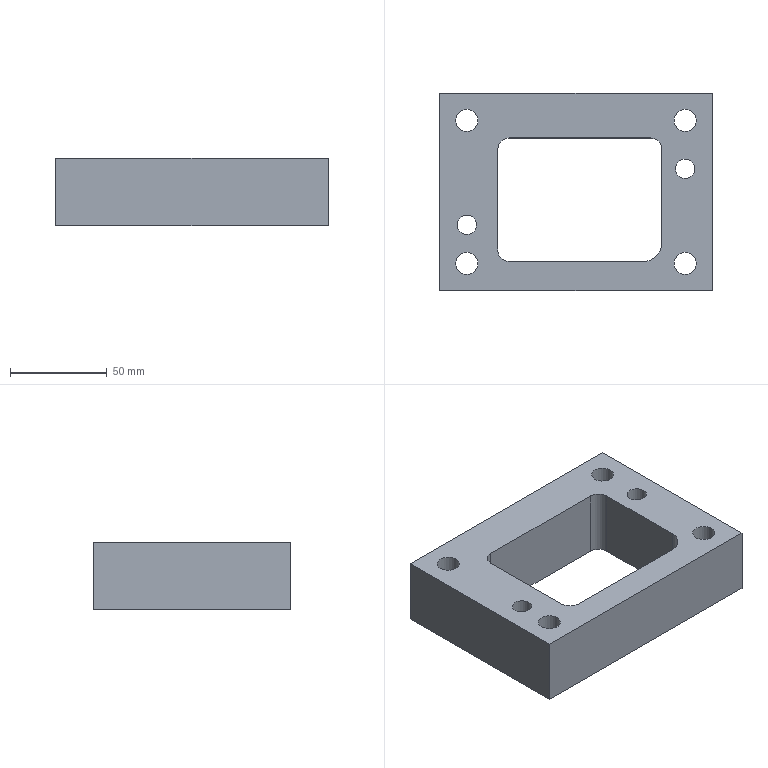Part | NX | features 7 2 | 1 solid | 32 faces | box 141 x 102 x 35 mm | volume 286562 mm3 | plane 16 | cylinder 16 | commonest cylinder face diameters 11.5 x4 18 x4 12 x3 10.001 x2 10.31 x2 20 x1
STEP:
#1=CARTESIAN_POINT('',(64.279,-375.95,69.));
#2=VERTEX_POINT('',#1);
#3=CARTESIAN_POINT('',(58.529,-375.95,69.));
#4=DIRECTION('',(0.,0.,-1.));
#5=DIRECTION('',(1.,0.,0.));
#6=AXIS2_PLACEMENT_3D('',#3,#4,#5);
#7=CIRCLE('',#6,5.75);
#8=EDGE_CURVE('',#2,#2,#7,.T.);
#9=ORIENTED_EDGE('',*,*,#8,.F.);
#10=EDGE_LOOP('',(#9));
#11=FACE_BOUND('',#10,.T.);
#12=CARTESIAN_POINT('',(67.529,-375.95,69.));
#13=VERTEX_POINT('',#12);
#14=CARTESIAN_POINT('',(58.529,-375.95,69.));
#15=DIRECTION('',(0.,0.,-1.));
#16=DIRECTION('',(1.,0.,0.));
#17=AXIS2_PLACEMENT_3D('',#14,#15,#16);
#18=CIRCLE('',#17,9.);
#19=EDGE_CURVE('',#13,#13,#18,.T.);
#20=ORIENTED_EDGE('',*,*,#19,.T.);
#21=EDGE_LOOP('',(#20));
#22=FACE_BOUND('',#21,.T.);
#23=CARTESIAN_POINT('',(58.529,-375.95,69.));
#24=DIRECTION('',(0.,0.,1.));
#25=DIRECTION('',(-1.,0.,0.));
#26=AXIS2_PLACEMENT_3D('',#23,#24,#25);
#27=PLANE('',#26);
#28=ADVANCED_FACE('',(#11,#22),#27,.F.);
#29=CARTESIAN_POINT('',(177.279,-449.95,69.));
#30=VERTEX_POINT('',#29);
#31=CARTESIAN_POINT('',(171.529,-449.95,69.));
#32=DIRECTION('',(0.,0.,-1.));
#33=DIRECTION('',(1.,0.,0.));
#34=AXIS2_PLACEMENT_3D('',#31,#32,#33);
#35=CIRCLE('',#34,5.75);
#36=EDGE_CURVE('',#30,#30,#35,.T.);
#37=ORIENTED_EDGE('',*,*,#36,.F.);
#38=EDGE_LOOP('',(#37));
#39=FACE_BOUND('',#38,.T.);
#40=CARTESIAN_POINT('',(180.529,-449.95,69.));
#41=VERTEX_POINT('',#40);
#42=CARTESIAN_POINT('',(171.529,-449.95,69.));
#43=DIRECTION('',(0.,0.,-1.));
#44=DIRECTION('',(1.,0.,0.));
#45=AXIS2_PLACEMENT_3D('',#42,#43,#44);
#46=CIRCLE('',#45,9.);
#47=EDGE_CURVE('',#41,#41,#46,.T.);
#48=ORIENTED_EDGE('',*,*,#47,.T.);
#49=EDGE_LOOP('',(#48));
#50=FACE_BOUND('',#49,.T.);
#51=CARTESIAN_POINT('',(171.529,-449.95,69.));
#52=DIRECTION('',(0.,0.,1.));
#53=DIRECTION('',(-1.,0.,0.));
#54=AXIS2_PLACEMENT_3D('',#51,#52,#53);
#55=PLANE('',#54);
#56=ADVANCED_FACE('',(#39,#50),#55,.F.);
#57=CARTESIAN_POINT('',(177.279,-375.95,69.));
#58=VERTEX_POINT('',#57);
#59=CARTESIAN_POINT('',(171.529,-375.95,69.));
#60=DIRECTION('',(0.,0.,-1.));
#61=DIRECTION('',(1.,0.,0.));
#62=AXIS2_PLACEMENT_3D('',#59,#60,#61);
#63=CIRCLE('',#62,5.75);
#64=EDGE_CURVE('',#58,#58,#63,.T.);
#65=ORIENTED_EDGE('',*,*,#64,.F.);
#66=EDGE_LOOP('',(#65));
#67=FACE_BOUND('',#66,.T.);
#68=CARTESIAN_POINT('',(180.529,-375.95,69.));
#69=VERTEX_POINT('',#68);
#70=CARTESIAN_POINT('',(171.529,-375.95,69.));
#71=DIRECTION('',(0.,0.,-1.));
#72=DIRECTION('',(1.,0.,0.));
#73=AXIS2_PLACEMENT_3D('',#70,#71,#72);
#74=CIRCLE('',#73,9.);
#75=EDGE_CURVE('',#69,#69,#74,.T.);
#76=ORIENTED_EDGE('',*,*,#75,.T.);
#77=EDGE_LOOP('',(#76));
#78=FACE_BOUND('',#77,.T.);
#79=CARTESIAN_POINT('',(171.529,-375.95,69.));
#80=DIRECTION('',(0.,0.,1.));
#81=DIRECTION('',(-1.,0.,0.));
#82=AXIS2_PLACEMENT_3D('',#79,#80,#81);
#83=PLANE('',#82);
#84=ADVANCED_FACE('',(#67,#78),#83,.F.);
#85=CARTESIAN_POINT('',(177.279,-449.95,91.));
#86=VERTEX_POINT('',#85);
#87=CARTESIAN_POINT('',(171.529,-449.95,91.));
#88=DIRECTION('',(0.,0.,-1.));
#89=DIRECTION('',(1.,0.,0.));
#90=AXIS2_PLACEMENT_3D('',#87,#88,#89);
#91=CIRCLE('',#90,5.75);
#92=EDGE_CURVE('',#86,#86,#91,.T.);
#93=ORIENTED_EDGE('',*,*,#92,.F.);
#94=EDGE_LOOP('',(#93));
#95=FACE_BOUND('',#94,.T.);
#96=ORIENTED_EDGE('',*,*,#36,.T.);
#97=EDGE_LOOP('',(#96));
#98=FACE_BOUND('',#97,.T.);
#99=CARTESIAN_POINT('',(171.529,-449.95,51.));
#100=DIRECTION('',(0.,0.,1.));
#101=DIRECTION('',(-1.,0.,0.));
#102=AXIS2_PLACEMENT_3D('',#99,#100,#101);
#103=CYLINDRICAL_SURFACE('',#102,5.75);
#104=ADVANCED_FACE('',(#95,#98),#103,.F.);
#105=CARTESIAN_POINT('',(64.279,-375.95,91.));
#106=VERTEX_POINT('',#105);
#107=CARTESIAN_POINT('',(58.529,-375.95,91.));
#108=DIRECTION('',(0.,0.,-1.));
#109=DIRECTION('',(1.,0.,0.));
#110=AXIS2_PLACEMENT_3D('',#107,#108,#109);
#111=CIRCLE('',#110,5.75);
#112=EDGE_CURVE('',#106,#106,#111,.T.);
#113=ORIENTED_EDGE('',*,*,#112,.F.);
#114=EDGE_LOOP('',(#113));
#115=FACE_BOUND('',#114,.T.);
#116=ORIENTED_EDGE('',*,*,#8,.T.);
#117=EDGE_LOOP('',(#116));
#118=FACE_BOUND('',#117,.T.);
#119=CARTESIAN_POINT('',(58.529,-375.95,51.));
#120=DIRECTION('',(0.,0.,1.));
#121=DIRECTION('',(-1.,0.,0.));
#122=AXIS2_PLACEMENT_3D('',#119,#120,#121);
#123=CYLINDRICAL_SURFACE('',#122,5.75);
#124=ADVANCED_FACE('',(#115,#118),#123,.F.);
#125=CARTESIAN_POINT('',(176.529,-400.95,66.));
#126=VERTEX_POINT('',#125);
#127=CARTESIAN_POINT('',(171.529,-400.95,66.));
#128=DIRECTION('',(0.,0.,-1.));
#129=DIRECTION('',(1.,0.,0.));
#130=AXIS2_PLACEMENT_3D('',#127,#128,#129);
#131=CIRCLE('',#130,5.);
#132=EDGE_CURVE('',#126,#126,#131,.T.);
#133=ORIENTED_EDGE('',*,*,#132,.T.);
#134=EDGE_LOOP('',(#133));
#135=FACE_BOUND('',#134,.T.);
#136=CARTESIAN_POINT('',(176.529,-400.95,91.));
#137=VERTEX_POINT('',#136);
#138=CARTESIAN_POINT('',(171.529,-400.95,91.));
#139=DIRECTION('',(0.,0.,1.));
#140=DIRECTION('',(1.,0.,0.));
#141=AXIS2_PLACEMENT_3D('',#138,#139,#140);
#142=CIRCLE('',#141,5.);
#143=EDGE_CURVE('',#137,#137,#142,.T.);
#144=ORIENTED_EDGE('',*,*,#143,.T.);
#145=EDGE_LOOP('',(#144));
#146=FACE_BOUND('',#145,.T.);
#147=CARTESIAN_POINT('',(171.529,-400.95,621.));
#148=DIRECTION('',(0.,0.,-1.));
#149=DIRECTION('',(1.,0.,0.));
#150=AXIS2_PLACEMENT_3D('',#147,#148,#149);
#151=CYLINDRICAL_SURFACE('',#150,5.);
#152=ADVANCED_FACE('',(#135,#146),#151,.F.);
#153=CARTESIAN_POINT('',(63.529,-429.95,66.));
#154=VERTEX_POINT('',#153);
#155=CARTESIAN_POINT('',(58.529,-429.95,66.));
#156=DIRECTION('',(0.,0.,-1.));
#157=DIRECTION('',(1.,0.,0.));
#158=AXIS2_PLACEMENT_3D('',#155,#156,#157);
#159=CIRCLE('',#158,5.);
#160=EDGE_CURVE('',#154,#154,#159,.T.);
#161=ORIENTED_EDGE('',*,*,#160,.T.);
#162=EDGE_LOOP('',(#161));
#163=FACE_BOUND('',#162,.T.);
#164=CARTESIAN_POINT('',(63.529,-429.95,91.));
#165=VERTEX_POINT('',#164);
#166=CARTESIAN_POINT('',(58.529,-429.95,91.));
#167=DIRECTION('',(0.,0.,1.));
#168=DIRECTION('',(1.,0.,0.));
#169=AXIS2_PLACEMENT_3D('',#166,#167,#168);
#170=CIRCLE('',#169,5.);
#171=EDGE_CURVE('',#165,#165,#170,.T.);
#172=ORIENTED_EDGE('',*,*,#171,.T.);
#173=EDGE_LOOP('',(#172));
#174=FACE_BOUND('',#173,.T.);
#175=CARTESIAN_POINT('',(58.529,-429.95,621.));
#176=DIRECTION('',(0.,0.,-1.));
#177=DIRECTION('',(1.,0.,0.));
#178=AXIS2_PLACEMENT_3D('',#175,#176,#177);
#179=CYLINDRICAL_SURFACE('',#178,5.);
#180=ADVANCED_FACE('',(#163,#174),#179,.F.);
#181=CARTESIAN_POINT('',(44.529,-463.95,56.));
#182=VERTEX_POINT('',#181);
#183=CARTESIAN_POINT('',(44.529,-463.95,91.));
#184=VERTEX_POINT('',#183);
#185=CARTESIAN_POINT('',(44.529,-463.95,6.933));
#186=DIRECTION('',(0.,0.,1.));
#187=VECTOR('',#186,1000.);
#188=LINE('',#185,#187);
#189=EDGE_CURVE('',#182,#184,#188,.T.);
#190=ORIENTED_EDGE('',*,*,#189,.F.);
#191=CARTESIAN_POINT('',(185.529,-463.95,56.));
#192=VERTEX_POINT('',#191);
#193=CARTESIAN_POINT('',(87.029,-463.95,56.));
#194=DIRECTION('',(-1.,0.,0.));
#195=VECTOR('',#194,1000.);
#196=LINE('',#193,#195);
#197=EDGE_CURVE('',#192,#182,#196,.T.);
#198=ORIENTED_EDGE('',*,*,#197,.F.);
#199=CARTESIAN_POINT('',(185.529,-463.95,91.));
#200=VERTEX_POINT('',#199);
#201=CARTESIAN_POINT('',(185.529,-463.95,6.933));
#202=DIRECTION('',(0.,0.,1.));
#203=VECTOR('',#202,1000.);
#204=LINE('',#201,#203);
#205=EDGE_CURVE('',#192,#200,#204,.T.);
#206=ORIENTED_EDGE('',*,*,#205,.T.);
#207=CARTESIAN_POINT('',(87.029,-463.95,91.));
#208=DIRECTION('',(1.,0.,0.));
#209=VECTOR('',#208,1000.);
#210=LINE('',#207,#209);
#211=EDGE_CURVE('',#184,#200,#210,.T.);
#212=ORIENTED_EDGE('',*,*,#211,.F.);
#213=EDGE_LOOP('',(#190,#198,#206,#212));
#214=FACE_BOUND('',#213,.T.);
#215=CARTESIAN_POINT('',(87.029,-463.95,6.933));
#216=DIRECTION('',(0.,-1.,0.));
#217=DIRECTION('',(0.,0.,-1.));
#218=AXIS2_PLACEMENT_3D('',#215,#216,#217);
#219=PLANE('',#218);
#220=ADVANCED_FACE('',(#214),#219,.T.);
#221=ORIENTED_EDGE('',*,*,#205,.F.);
#222=CARTESIAN_POINT('',(185.529,-361.95,56.));
#223=VERTEX_POINT('',#222);
#224=CARTESIAN_POINT('',(185.529,-411.95,56.));
#225=DIRECTION('',(0.,-1.,0.));
#226=VECTOR('',#225,1000.);
#227=LINE('',#224,#226);
#228=EDGE_CURVE('',#223,#192,#227,.T.);
#229=ORIENTED_EDGE('',*,*,#228,.F.);
#230=CARTESIAN_POINT('',(185.529,-361.95,91.));
#231=VERTEX_POINT('',#230);
#232=CARTESIAN_POINT('',(185.529,-361.95,6.933));
#233=DIRECTION('',(0.,0.,1.));
#234=VECTOR('',#233,1000.);
#235=LINE('',#232,#234);
#236=EDGE_CURVE('',#223,#231,#235,.T.);
#237=ORIENTED_EDGE('',*,*,#236,.T.);
#238=CARTESIAN_POINT('',(185.529,-411.95,91.));
#239=DIRECTION('',(0.,1.,0.));
#240=VECTOR('',#239,1000.);
#241=LINE('',#238,#240);
#242=EDGE_CURVE('',#200,#231,#241,.T.);
#243=ORIENTED_EDGE('',*,*,#242,.F.);
#244=EDGE_LOOP('',(#221,#229,#237,#243));
#245=FACE_BOUND('',#244,.T.);
#246=CARTESIAN_POINT('',(185.529,-411.95,6.933));
#247=DIRECTION('',(1.,0.,0.));
#248=DIRECTION('',(0.,0.,1.));
#249=AXIS2_PLACEMENT_3D('',#246,#247,#248);
#250=PLANE('',#249);
#251=ADVANCED_FACE('',(#245),#250,.T.);
#252=ORIENTED_EDGE('',*,*,#236,.F.);
#253=CARTESIAN_POINT('',(44.529,-361.95,56.));
#254=VERTEX_POINT('',#253);
#255=CARTESIAN_POINT('',(87.029,-361.95,56.));
#256=DIRECTION('',(1.,0.,0.));
#257=VECTOR('',#256,1000.);
#258=LINE('',#255,#257);
#259=EDGE_CURVE('',#254,#223,#258,.T.);
#260=ORIENTED_EDGE('',*,*,#259,.F.);
#261=CARTESIAN_POINT('',(44.529,-361.95,91.));
#262=VERTEX_POINT('',#261);
#263=CARTESIAN_POINT('',(44.529,-361.95,6.933));
#264=DIRECTION('',(0.,0.,1.));
#265=VECTOR('',#264,1000.);
#266=LINE('',#263,#265);
#267=EDGE_CURVE('',#254,#262,#266,.T.);
#268=ORIENTED_EDGE('',*,*,#267,.T.);
#269=CARTESIAN_POINT('',(87.029,-361.95,91.));
#270=DIRECTION('',(-1.,0.,0.));
#271=VECTOR('',#270,1000.);
#272=LINE('',#269,#271);
#273=EDGE_CURVE('',#231,#262,#272,.T.);
#274=ORIENTED_EDGE('',*,*,#273,.F.);
#275=EDGE_LOOP('',(#252,#260,#268,#274));
#276=FACE_BOUND('',#275,.T.);
#277=CARTESIAN_POINT('',(87.029,-361.95,6.933));
#278=DIRECTION('',(0.,1.,0.));
#279=DIRECTION('',(0.,0.,1.));
#280=AXIS2_PLACEMENT_3D('',#277,#278,#279);
#281=PLANE('',#280);
#282=ADVANCED_FACE('',(#276),#281,.T.);
#283=ORIENTED_EDGE('',*,*,#267,.F.);
#284=CARTESIAN_POINT('',(44.529,-411.95,56.));
#285=DIRECTION('',(0.,1.,0.));
#286=VECTOR('',#285,1000.);
#287=LINE('',#284,#286);
#288=EDGE_CURVE('',#182,#254,#287,.T.);
#289=ORIENTED_EDGE('',*,*,#288,.F.);
#290=ORIENTED_EDGE('',*,*,#189,.T.);
#291=CARTESIAN_POINT('',(44.529,-411.95,91.));
#292=DIRECTION('',(0.,-1.,0.));
#293=VECTOR('',#292,1000.);
#294=LINE('',#291,#293);
#295=EDGE_CURVE('',#262,#184,#294,.T.);
#296=ORIENTED_EDGE('',*,*,#295,.F.);
#297=EDGE_LOOP('',(#283,#289,#290,#296));
#298=FACE_BOUND('',#297,.T.);
#299=CARTESIAN_POINT('',(44.529,-411.95,6.933));
#300=DIRECTION('',(-1.,0.,0.));
#301=DIRECTION('',(0.,0.,-1.));
#302=AXIS2_PLACEMENT_3D('',#299,#300,#301);
#303=PLANE('',#302);
#304=ADVANCED_FACE('',(#298),#303,.T.);
#305=ORIENTED_EDGE('',*,*,#19,.F.);
#306=EDGE_LOOP('',(#305));
#307=FACE_BOUND('',#306,.T.);
#308=CARTESIAN_POINT('',(49.529,-375.95,56.));
#309=VERTEX_POINT('',#308);
#310=CARTESIAN_POINT('',(58.529,-375.95,56.));
#311=DIRECTION('',(0.,0.,-1.));
#312=DIRECTION('',(-1.,0.,0.));
#313=AXIS2_PLACEMENT_3D('',#310,#311,#312);
#314=CIRCLE('',#313,9.);
#315=EDGE_CURVE('',#309,#309,#314,.T.);
#316=ORIENTED_EDGE('',*,*,#315,.T.);
#317=EDGE_LOOP('',(#316));
#318=FACE_BOUND('',#317,.T.);
#319=CARTESIAN_POINT('',(58.529,-375.95,56.));
#320=DIRECTION('',(0.,0.,1.));
#321=DIRECTION('',(-1.,0.,0.));
#322=AXIS2_PLACEMENT_3D('',#319,#320,#321);
#323=CYLINDRICAL_SURFACE('',#322,9.);
#324=ADVANCED_FACE('',(#307,#318),#323,.F.);
#325=ORIENTED_EDGE('',*,*,#47,.F.);
#326=EDGE_LOOP('',(#325));
#327=FACE_BOUND('',#326,.T.);
#328=CARTESIAN_POINT('',(162.529,-449.95,56.));
#329=VERTEX_POINT('',#328);
#330=CARTESIAN_POINT('',(171.529,-449.95,56.));
#331=DIRECTION('',(0.,0.,-1.));
#332=DIRECTION('',(-1.,0.,0.));
#333=AXIS2_PLACEMENT_3D('',#330,#331,#332);
#334=CIRCLE('',#333,9.);
#335=EDGE_CURVE('',#329,#329,#334,.T.);
#336=ORIENTED_EDGE('',*,*,#335,.T.);
#337=EDGE_LOOP('',(#336));
#338=FACE_BOUND('',#337,.T.);
#339=CARTESIAN_POINT('',(171.529,-449.95,56.));
#340=DIRECTION('',(0.,0.,1.));
#341=DIRECTION('',(-1.,0.,0.));
#342=AXIS2_PLACEMENT_3D('',#339,#340,#341);
#343=CYLINDRICAL_SURFACE('',#342,9.);
#344=ADVANCED_FACE('',(#327,#338),#343,.F.);
#345=CARTESIAN_POINT('',(159.529,-439.,91.));
#346=VERTEX_POINT('',#345);
#347=CARTESIAN_POINT('',(149.529,-449.,91.));
#348=VERTEX_POINT('',#347);
#349=CARTESIAN_POINT('',(149.529,-439.,91.));
#350=DIRECTION('',(0.,0.,-1.));
#351=DIRECTION('',(1.,0.,0.));
#352=AXIS2_PLACEMENT_3D('',#349,#350,#351);
#353=CIRCLE('',#352,10.);
#354=EDGE_CURVE('',#346,#348,#353,.T.);
#355=ORIENTED_EDGE('',*,*,#354,.F.);
#356=CARTESIAN_POINT('',(159.529,-439.,56.));
#357=VERTEX_POINT('',#356);
#358=CARTESIAN_POINT('',(159.529,-439.,19.186));
#359=DIRECTION('',(0.,0.,1.));
#360=VECTOR('',#359,1000.);
#361=LINE('',#358,#360);
#362=EDGE_CURVE('',#357,#346,#361,.T.);
#363=ORIENTED_EDGE('',*,*,#362,.F.);
#364=CARTESIAN_POINT('',(149.529,-449.,56.));
#365=VERTEX_POINT('',#364);
#366=CARTESIAN_POINT('',(149.529,-439.,56.));
#367=DIRECTION('',(0.,0.,1.));
#368=DIRECTION('',(-1.,0.,0.));
#369=AXIS2_PLACEMENT_3D('',#366,#367,#368);
#370=CIRCLE('',#369,10.);
#371=EDGE_CURVE('',#365,#357,#370,.T.);
#372=ORIENTED_EDGE('',*,*,#371,.F.);
#373=CARTESIAN_POINT('',(149.529,-449.,19.186));
#374=DIRECTION('',(0.,0.,-1.));
#375=VECTOR('',#374,1000.);
#376=LINE('',#373,#375);
#377=EDGE_CURVE('',#348,#365,#376,.T.);
#378=ORIENTED_EDGE('',*,*,#377,.F.);
#379=EDGE_LOOP('',(#355,#363,#372,#378));
#380=FACE_BOUND('',#379,.T.);
#381=CARTESIAN_POINT('',(149.529,-439.,19.186));
#382=DIRECTION('',(0.,0.,-1.));
#383=DIRECTION('',(1.,0.,0.));
#384=AXIS2_PLACEMENT_3D('',#381,#382,#383);
#385=CYLINDRICAL_SURFACE('',#384,10.);
#386=ADVANCED_FACE('',(#380),#385,.F.);
#387=CARTESIAN_POINT('',(80.529,-449.,91.));
#388=VERTEX_POINT('',#387);
#389=CARTESIAN_POINT('',(116.864,-449.,91.));
#390=DIRECTION('',(1.,0.,0.));
#391=VECTOR('',#390,1000.);
#392=LINE('',#389,#391);
#393=EDGE_CURVE('',#388,#348,#392,.T.);
#394=ORIENTED_EDGE('',*,*,#393,.T.);
#395=ORIENTED_EDGE('',*,*,#377,.T.);
#396=CARTESIAN_POINT('',(80.529,-449.,56.));
#397=VERTEX_POINT('',#396);
#398=CARTESIAN_POINT('',(116.864,-449.,56.));
#399=DIRECTION('',(-1.,0.,0.));
#400=VECTOR('',#399,1000.);
#401=LINE('',#398,#400);
#402=EDGE_CURVE('',#365,#397,#401,.T.);
#403=ORIENTED_EDGE('',*,*,#402,.T.);
#404=CARTESIAN_POINT('',(80.529,-449.,91.));
#405=DIRECTION('',(0.,0.,1.));
#406=VECTOR('',#405,1000.);
#407=LINE('',#404,#406);
#408=EDGE_CURVE('',#397,#388,#407,.T.);
#409=ORIENTED_EDGE('',*,*,#408,.T.);
#410=EDGE_LOOP('',(#394,#395,#403,#409));
#411=FACE_BOUND('',#410,.T.);
#412=CARTESIAN_POINT('',(116.864,-449.,19.186));
#413=DIRECTION('',(0.,-1.,0.));
#414=DIRECTION('',(0.,0.,1.));
#415=AXIS2_PLACEMENT_3D('',#412,#413,#414);
#416=PLANE('',#415);
#417=ADVANCED_FACE('',(#411),#416,.F.);
#418=CARTESIAN_POINT('',(74.529,-443.,91.));
#419=VERTEX_POINT('',#418);
#420=CARTESIAN_POINT('',(80.529,-443.,91.));
#421=DIRECTION('',(0.,0.,-1.));
#422=DIRECTION('',(1.,0.,0.));
#423=AXIS2_PLACEMENT_3D('',#420,#421,#422);
#424=CIRCLE('',#423,6.);
#425=EDGE_CURVE('',#388,#419,#424,.T.);
#426=ORIENTED_EDGE('',*,*,#425,.F.);
#427=ORIENTED_EDGE('',*,*,#408,.F.);
#428=CARTESIAN_POINT('',(74.529,-443.,56.));
#429=VERTEX_POINT('',#428);
#430=CARTESIAN_POINT('',(80.529,-443.,56.));
#431=DIRECTION('',(0.,0.,1.));
#432=DIRECTION('',(-1.,0.,0.));
#433=AXIS2_PLACEMENT_3D('',#430,#431,#432);
#434=CIRCLE('',#433,6.);
#435=EDGE_CURVE('',#429,#397,#434,.T.);
#436=ORIENTED_EDGE('',*,*,#435,.F.);
#437=CARTESIAN_POINT('',(74.529,-443.,56.));
#438=DIRECTION('',(0.,0.,-1.));
#439=VECTOR('',#438,1000.);
#440=LINE('',#437,#439);
#441=EDGE_CURVE('',#419,#429,#440,.T.);
#442=ORIENTED_EDGE('',*,*,#441,.F.);
#443=EDGE_LOOP('',(#426,#427,#436,#442));
#444=FACE_BOUND('',#443,.T.);
#445=CARTESIAN_POINT('',(80.529,-443.,19.186));
#446=DIRECTION('',(0.,0.,1.));
#447=DIRECTION('',(-1.,0.,0.));
#448=AXIS2_PLACEMENT_3D('',#445,#446,#447);
#449=CYLINDRICAL_SURFACE('',#448,6.);
#450=ADVANCED_FACE('',(#444),#449,.F.);
#451=CARTESIAN_POINT('',(74.529,-391.,56.));
#452=VERTEX_POINT('',#451);
#453=CARTESIAN_POINT('',(74.529,-424.225,56.));
#454=DIRECTION('',(0.,-1.,0.));
#455=VECTOR('',#454,1000.);
#456=LINE('',#453,#455);
#457=EDGE_CURVE('',#452,#429,#456,.T.);
#458=ORIENTED_EDGE('',*,*,#457,.F.);
#459=CARTESIAN_POINT('',(74.529,-391.,91.));
#460=VERTEX_POINT('',#459);
#461=CARTESIAN_POINT('',(74.529,-391.,91.));
#462=DIRECTION('',(0.,0.,1.));
#463=VECTOR('',#462,1000.);
#464=LINE('',#461,#463);
#465=EDGE_CURVE('',#452,#460,#464,.T.);
#466=ORIENTED_EDGE('',*,*,#465,.T.);
#467=CARTESIAN_POINT('',(74.529,-424.225,91.));
#468=DIRECTION('',(0.,-1.,0.));
#469=VECTOR('',#468,1000.);
#470=LINE('',#467,#469);
#471=EDGE_CURVE('',#460,#419,#470,.T.);
#472=ORIENTED_EDGE('',*,*,#471,.T.);
#473=ORIENTED_EDGE('',*,*,#441,.T.);
#474=EDGE_LOOP('',(#458,#466,#472,#473));
#475=FACE_BOUND('',#474,.T.);
#476=CARTESIAN_POINT('',(74.529,-424.225,19.186));
#477=DIRECTION('',(-1.,0.,0.));
#478=DIRECTION('',(0.,0.,-1.));
#479=AXIS2_PLACEMENT_3D('',#476,#477,#478);
#480=PLANE('',#479);
#481=ADVANCED_FACE('',(#475),#480,.F.);
#482=CARTESIAN_POINT('',(80.529,-385.,56.));
#483=VERTEX_POINT('',#482);
#484=CARTESIAN_POINT('',(80.529,-391.,56.));
#485=DIRECTION('',(0.,0.,1.));
#486=DIRECTION('',(-1.,0.,0.));
#487=AXIS2_PLACEMENT_3D('',#484,#485,#486);
#488=CIRCLE('',#487,6.);
#489=EDGE_CURVE('',#483,#452,#488,.T.);
#490=ORIENTED_EDGE('',*,*,#489,.F.);
#491=CARTESIAN_POINT('',(80.529,-385.,91.));
#492=VERTEX_POINT('',#491);
#493=CARTESIAN_POINT('',(80.529,-385.,56.));
#494=DIRECTION('',(0.,0.,-1.));
#495=VECTOR('',#494,1000.);
#496=LINE('',#493,#495);
#497=EDGE_CURVE('',#492,#483,#496,.T.);
#498=ORIENTED_EDGE('',*,*,#497,.F.);
#499=CARTESIAN_POINT('',(80.529,-391.,91.));
#500=DIRECTION('',(0.,0.,-1.));
#501=DIRECTION('',(1.,0.,0.));
#502=AXIS2_PLACEMENT_3D('',#499,#500,#501);
#503=CIRCLE('',#502,6.);
#504=EDGE_CURVE('',#460,#492,#503,.T.);
#505=ORIENTED_EDGE('',*,*,#504,.F.);
#506=ORIENTED_EDGE('',*,*,#465,.F.);
#507=EDGE_LOOP('',(#490,#498,#505,#506));
#508=FACE_BOUND('',#507,.T.);
#509=CARTESIAN_POINT('',(80.529,-391.,19.186));
#510=DIRECTION('',(0.,0.,-1.));
#511=DIRECTION('',(1.,0.,0.));
#512=AXIS2_PLACEMENT_3D('',#509,#510,#511);
#513=CYLINDRICAL_SURFACE('',#512,6.);
#514=ADVANCED_FACE('',(#508),#513,.F.);
#515=CARTESIAN_POINT('',(153.529,-385.,56.));
#516=VERTEX_POINT('',#515);
#517=CARTESIAN_POINT('',(116.864,-385.,56.));
#518=DIRECTION('',(-1.,0.,0.));
#519=VECTOR('',#518,1000.);
#520=LINE('',#517,#519);
#521=EDGE_CURVE('',#516,#483,#520,.T.);
#522=ORIENTED_EDGE('',*,*,#521,.F.);
#523=CARTESIAN_POINT('',(153.529,-385.,91.));
#524=VERTEX_POINT('',#523);
#525=CARTESIAN_POINT('',(153.529,-385.,91.));
#526=DIRECTION('',(0.,0.,1.));
#527=VECTOR('',#526,1000.);
#528=LINE('',#525,#527);
#529=EDGE_CURVE('',#516,#524,#528,.T.);
#530=ORIENTED_EDGE('',*,*,#529,.T.);
#531=CARTESIAN_POINT('',(116.864,-385.,91.));
#532=DIRECTION('',(-1.,0.,0.));
#533=VECTOR('',#532,1000.);
#534=LINE('',#531,#533);
#535=EDGE_CURVE('',#524,#492,#534,.T.);
#536=ORIENTED_EDGE('',*,*,#535,.T.);
#537=ORIENTED_EDGE('',*,*,#497,.T.);
#538=EDGE_LOOP('',(#522,#530,#536,#537));
#539=FACE_BOUND('',#538,.T.);
#540=CARTESIAN_POINT('',(116.864,-385.,19.186));
#541=DIRECTION('',(0.,1.,0.));
#542=DIRECTION('',(0.,0.,-1.));
#543=AXIS2_PLACEMENT_3D('',#540,#541,#542);
#544=PLANE('',#543);
#545=ADVANCED_FACE('',(#539),#544,.F.);
#546=CARTESIAN_POINT('',(159.529,-391.,91.));
#547=VERTEX_POINT('',#546);
#548=CARTESIAN_POINT('',(153.529,-391.,91.));
#549=DIRECTION('',(0.,0.,-1.));
#550=DIRECTION('',(1.,0.,0.));
#551=AXIS2_PLACEMENT_3D('',#548,#549,#550);
#552=CIRCLE('',#551,6.);
#553=EDGE_CURVE('',#524,#547,#552,.T.);
#554=ORIENTED_EDGE('',*,*,#553,.F.);
#555=ORIENTED_EDGE('',*,*,#529,.F.);
#556=CARTESIAN_POINT('',(159.529,-391.,56.));
#557=VERTEX_POINT('',#556);
#558=CARTESIAN_POINT('',(153.529,-391.,56.));
#559=DIRECTION('',(0.,0.,1.));
#560=DIRECTION('',(-1.,0.,0.));
#561=AXIS2_PLACEMENT_3D('',#558,#559,#560);
#562=CIRCLE('',#561,6.);
#563=EDGE_CURVE('',#557,#516,#562,.T.);
#564=ORIENTED_EDGE('',*,*,#563,.F.);
#565=CARTESIAN_POINT('',(159.529,-391.,56.));
#566=DIRECTION('',(0.,0.,-1.));
#567=VECTOR('',#566,1000.);
#568=LINE('',#565,#567);
#569=EDGE_CURVE('',#547,#557,#568,.T.);
#570=ORIENTED_EDGE('',*,*,#569,.F.);
#571=EDGE_LOOP('',(#554,#555,#564,#570));
#572=FACE_BOUND('',#571,.T.);
#573=CARTESIAN_POINT('',(153.529,-391.,19.186));
#574=DIRECTION('',(0.,0.,1.));
#575=DIRECTION('',(-1.,0.,0.));
#576=AXIS2_PLACEMENT_3D('',#573,#574,#575);
#577=CYLINDRICAL_SURFACE('',#576,6.);
#578=ADVANCED_FACE('',(#572),#577,.F.);
#579=CARTESIAN_POINT('',(159.529,-424.225,56.));
#580=DIRECTION('',(0.,1.,0.));
#581=VECTOR('',#580,1000.);
#582=LINE('',#579,#581);
#583=EDGE_CURVE('',#357,#557,#582,.T.);
#584=ORIENTED_EDGE('',*,*,#583,.F.);
#585=ORIENTED_EDGE('',*,*,#362,.T.);
#586=CARTESIAN_POINT('',(159.529,-424.225,91.));
#587=DIRECTION('',(0.,1.,0.));
#588=VECTOR('',#587,1000.);
#589=LINE('',#586,#588);
#590=EDGE_CURVE('',#346,#547,#589,.T.);
#591=ORIENTED_EDGE('',*,*,#590,.T.);
#592=ORIENTED_EDGE('',*,*,#569,.T.);
#593=EDGE_LOOP('',(#584,#585,#591,#592));
#594=FACE_BOUND('',#593,.T.);
#595=CARTESIAN_POINT('',(159.529,-424.225,19.186));
#596=DIRECTION('',(1.,0.,0.));
#597=DIRECTION('',(0.,0.,1.));
#598=AXIS2_PLACEMENT_3D('',#595,#596,#597);
#599=PLANE('',#598);
#600=ADVANCED_FACE('',(#594),#599,.F.);
#601=ORIENTED_EDGE('',*,*,#75,.F.);
#602=EDGE_LOOP('',(#601));
#603=FACE_BOUND('',#602,.T.);
#604=CARTESIAN_POINT('',(162.529,-375.95,56.));
#605=VERTEX_POINT('',#604);
#606=CARTESIAN_POINT('',(171.529,-375.95,56.));
#607=DIRECTION('',(0.,0.,-1.));
#608=DIRECTION('',(-1.,0.,0.));
#609=AXIS2_PLACEMENT_3D('',#606,#607,#608);
#610=CIRCLE('',#609,9.);
#611=EDGE_CURVE('',#605,#605,#610,.T.);
#612=ORIENTED_EDGE('',*,*,#611,.T.);
#613=EDGE_LOOP('',(#612));
#614=FACE_BOUND('',#613,.T.);
#615=CARTESIAN_POINT('',(171.529,-375.95,56.));
#616=DIRECTION('',(0.,0.,1.));
#617=DIRECTION('',(-1.,0.,0.));
#618=AXIS2_PLACEMENT_3D('',#615,#616,#617);
#619=CYLINDRICAL_SURFACE('',#618,9.);
#620=ADVANCED_FACE('',(#603,#614),#619,.F.);
#621=CARTESIAN_POINT('',(176.684,-400.95,56.));
#622=VERTEX_POINT('',#621);
#623=CARTESIAN_POINT('',(171.529,-400.95,56.));
#624=DIRECTION('',(0.,0.,1.));
#625=DIRECTION('',(1.,0.,0.));
#626=AXIS2_PLACEMENT_3D('',#623,#624,#625);
#627=CIRCLE('',#626,5.155);
#628=EDGE_CURVE('',#622,#622,#627,.T.);
#629=ORIENTED_EDGE('',*,*,#628,.T.);
#630=EDGE_LOOP('',(#629));
#631=FACE_BOUND('',#630,.T.);
#632=CARTESIAN_POINT('',(63.684,-429.95,56.));
#633=VERTEX_POINT('',#632);
#634=CARTESIAN_POINT('',(58.529,-429.95,56.));
#635=DIRECTION('',(0.,0.,1.));
#636=DIRECTION('',(1.,0.,0.));
#637=AXIS2_PLACEMENT_3D('',#634,#635,#636);
#638=CIRCLE('',#637,5.155);
#639=EDGE_CURVE('',#633,#633,#638,.T.);
#640=ORIENTED_EDGE('',*,*,#639,.T.);
#641=EDGE_LOOP('',(#640));
#642=FACE_BOUND('',#641,.T.);
#643=CARTESIAN_POINT('',(49.529,-449.95,56.));
#644=VERTEX_POINT('',#643);
#645=CARTESIAN_POINT('',(58.529,-449.95,56.));
#646=DIRECTION('',(0.,0.,-1.));
#647=DIRECTION('',(-1.,0.,0.));
#648=AXIS2_PLACEMENT_3D('',#645,#646,#647);
#649=CIRCLE('',#648,9.);
#650=EDGE_CURVE('',#644,#644,#649,.T.);
#651=ORIENTED_EDGE('',*,*,#650,.F.);
#652=EDGE_LOOP('',(#651));
#653=FACE_BOUND('',#652,.T.);
#654=ORIENTED_EDGE('',*,*,#611,.F.);
#655=EDGE_LOOP('',(#654));
#656=FACE_BOUND('',#655,.T.);
#657=ORIENTED_EDGE('',*,*,#583,.T.);
#658=ORIENTED_EDGE('',*,*,#563,.T.);
#659=ORIENTED_EDGE('',*,*,#521,.T.);
#660=ORIENTED_EDGE('',*,*,#489,.T.);
#661=ORIENTED_EDGE('',*,*,#457,.T.);
#662=ORIENTED_EDGE('',*,*,#435,.T.);
#663=ORIENTED_EDGE('',*,*,#402,.F.);
#664=ORIENTED_EDGE('',*,*,#371,.T.);
#665=EDGE_LOOP('',(#657,#658,#659,#660,#661,#662,#663,#664));
#666=FACE_BOUND('',#665,.T.);
#667=ORIENTED_EDGE('',*,*,#335,.F.);
#668=EDGE_LOOP('',(#667));
#669=FACE_BOUND('',#668,.T.);
#670=ORIENTED_EDGE('',*,*,#315,.F.);
#671=EDGE_LOOP('',(#670));
#672=FACE_BOUND('',#671,.T.);
#673=ORIENTED_EDGE('',*,*,#288,.T.);
#674=ORIENTED_EDGE('',*,*,#259,.T.);
#675=ORIENTED_EDGE('',*,*,#228,.T.);
#676=ORIENTED_EDGE('',*,*,#197,.T.);
#677=EDGE_LOOP('',(#673,#674,#675,#676));
#678=FACE_BOUND('',#677,.T.);
#679=CARTESIAN_POINT('',(-89.971,-226.95,56.));
#680=DIRECTION('',(0.,0.,-1.));
#681=DIRECTION('',(1.,0.,0.));
#682=AXIS2_PLACEMENT_3D('',#679,#680,#681);
#683=PLANE('',#682);
#684=ADVANCED_FACE('',(#631,#642,#653,#656,#666,#669,#672,#678),#683,.T.);
#685=CARTESIAN_POINT('',(177.279,-375.95,91.));
#686=VERTEX_POINT('',#685);
#687=CARTESIAN_POINT('',(171.529,-375.95,91.));
#688=DIRECTION('',(0.,0.,1.));
#689=DIRECTION('',(1.,0.,0.));
#690=AXIS2_PLACEMENT_3D('',#687,#688,#689);
#691=CIRCLE('',#690,5.75);
#692=EDGE_CURVE('',#686,#686,#691,.T.);
#693=ORIENTED_EDGE('',*,*,#692,.T.);
#694=EDGE_LOOP('',(#693));
#695=FACE_BOUND('',#694,.T.);
#696=ORIENTED_EDGE('',*,*,#64,.T.);
#697=EDGE_LOOP('',(#696));
#698=FACE_BOUND('',#697,.T.);
#699=CARTESIAN_POINT('',(171.529,-375.95,51.));
#700=DIRECTION('',(0.,0.,1.));
#701=DIRECTION('',(-1.,0.,0.));
#702=AXIS2_PLACEMENT_3D('',#699,#700,#701);
#703=CYLINDRICAL_SURFACE('',#702,5.75);
#704=ADVANCED_FACE('',(#695,#698),#703,.F.);
#705=CARTESIAN_POINT('',(64.279,-449.95,91.));
#706=VERTEX_POINT('',#705);
#707=CARTESIAN_POINT('',(58.529,-449.95,91.));
#708=DIRECTION('',(0.,0.,1.));
#709=DIRECTION('',(1.,0.,0.));
#710=AXIS2_PLACEMENT_3D('',#707,#708,#709);
#711=CIRCLE('',#710,5.75);
#712=EDGE_CURVE('',#706,#706,#711,.T.);
#713=ORIENTED_EDGE('',*,*,#712,.F.);
#714=EDGE_LOOP('',(#713));
#715=FACE_BOUND('',#714,.T.);
#716=ORIENTED_EDGE('',*,*,#692,.F.);
#717=EDGE_LOOP('',(#716));
#718=FACE_BOUND('',#717,.T.);
#719=ORIENTED_EDGE('',*,*,#471,.F.);
#720=ORIENTED_EDGE('',*,*,#504,.T.);
#721=ORIENTED_EDGE('',*,*,#535,.F.);
#722=ORIENTED_EDGE('',*,*,#553,.T.);
#723=ORIENTED_EDGE('',*,*,#590,.F.);
#724=ORIENTED_EDGE('',*,*,#354,.T.);
#725=ORIENTED_EDGE('',*,*,#393,.F.);
#726=ORIENTED_EDGE('',*,*,#425,.T.);
#727=EDGE_LOOP('',(#719,#720,#721,#722,#723,#724,#725,#726));
#728=FACE_BOUND('',#727,.T.);
#729=ORIENTED_EDGE('',*,*,#171,.F.);
#730=EDGE_LOOP('',(#729));
#731=FACE_BOUND('',#730,.T.);
#732=ORIENTED_EDGE('',*,*,#112,.T.);
#733=EDGE_LOOP('',(#732));
#734=FACE_BOUND('',#733,.T.);
#735=ORIENTED_EDGE('',*,*,#211,.T.);
#736=ORIENTED_EDGE('',*,*,#242,.T.);
#737=ORIENTED_EDGE('',*,*,#273,.T.);
#738=ORIENTED_EDGE('',*,*,#295,.T.);
#739=EDGE_LOOP('',(#735,#736,#737,#738));
#740=FACE_BOUND('',#739,.T.);
#741=ORIENTED_EDGE('',*,*,#92,.T.);
#742=EDGE_LOOP('',(#741));
#743=FACE_BOUND('',#742,.T.);
#744=ORIENTED_EDGE('',*,*,#143,.F.);
#745=EDGE_LOOP('',(#744));
#746=FACE_BOUND('',#745,.T.);
#747=CARTESIAN_POINT('',(87.029,-411.95,91.));
#748=DIRECTION('',(0.,0.,1.));
#749=DIRECTION('',(-1.,0.,0.));
#750=AXIS2_PLACEMENT_3D('',#747,#748,#749);
#751=PLANE('',#750);
#752=ADVANCED_FACE('',(#715,#718,#728,#731,#734,#740,#743,#746),#751,.T.);
#753=CARTESIAN_POINT('',(64.279,-449.95,69.));
#754=VERTEX_POINT('',#753);
#755=CARTESIAN_POINT('',(58.529,-449.95,69.));
#756=DIRECTION('',(0.,0.,-1.));
#757=DIRECTION('',(1.,0.,0.));
#758=AXIS2_PLACEMENT_3D('',#755,#756,#757);
#759=CIRCLE('',#758,5.75);
#760=EDGE_CURVE('',#754,#754,#759,.T.);
#761=ORIENTED_EDGE('',*,*,#760,.F.);
#762=EDGE_LOOP('',(#761));
#763=FACE_BOUND('',#762,.T.);
#764=CARTESIAN_POINT('',(67.529,-449.95,69.));
#765=VERTEX_POINT('',#764);
#766=CARTESIAN_POINT('',(58.529,-449.95,69.));
#767=DIRECTION('',(0.,0.,-1.));
#768=DIRECTION('',(1.,0.,0.));
#769=AXIS2_PLACEMENT_3D('',#766,#767,#768);
#770=CIRCLE('',#769,9.);
#771=EDGE_CURVE('',#765,#765,#770,.T.);
#772=ORIENTED_EDGE('',*,*,#771,.T.);
#773=EDGE_LOOP('',(#772));
#774=FACE_BOUND('',#773,.T.);
#775=CARTESIAN_POINT('',(58.529,-449.95,69.));
#776=DIRECTION('',(0.,0.,1.));
#777=DIRECTION('',(-1.,0.,0.));
#778=AXIS2_PLACEMENT_3D('',#775,#776,#777);
#779=PLANE('',#778);
#780=ADVANCED_FACE('',(#763,#774),#779,.F.);
#781=ORIENTED_EDGE('',*,*,#771,.F.);
#782=EDGE_LOOP('',(#781));
#783=FACE_BOUND('',#782,.T.);
#784=ORIENTED_EDGE('',*,*,#650,.T.);
#785=EDGE_LOOP('',(#784));
#786=FACE_BOUND('',#785,.T.);
#787=CARTESIAN_POINT('',(58.529,-449.95,56.));
#788=DIRECTION('',(0.,0.,1.));
#789=DIRECTION('',(-1.,0.,0.));
#790=AXIS2_PLACEMENT_3D('',#787,#788,#789);
#791=CYLINDRICAL_SURFACE('',#790,9.);
#792=ADVANCED_FACE('',(#783,#786),#791,.F.);
#793=ORIENTED_EDGE('',*,*,#712,.T.);
#794=EDGE_LOOP('',(#793));
#795=FACE_BOUND('',#794,.T.);
#796=ORIENTED_EDGE('',*,*,#760,.T.);
#797=EDGE_LOOP('',(#796));
#798=FACE_BOUND('',#797,.T.);
#799=CARTESIAN_POINT('',(58.529,-449.95,51.));
#800=DIRECTION('',(0.,0.,1.));
#801=DIRECTION('',(-1.,0.,0.));
#802=AXIS2_PLACEMENT_3D('',#799,#800,#801);
#803=CYLINDRICAL_SURFACE('',#802,5.75);
#804=ADVANCED_FACE('',(#795,#798),#803,.F.);
#805=CARTESIAN_POINT('',(63.684,-429.95,66.));
#806=VERTEX_POINT('',#805);
#807=CARTESIAN_POINT('',(58.529,-429.95,66.));
#808=DIRECTION('',(0.,0.,-1.));
#809=DIRECTION('',(1.,0.,0.));
#810=AXIS2_PLACEMENT_3D('',#807,#808,#809);
#811=CIRCLE('',#810,5.155);
#812=EDGE_CURVE('',#806,#806,#811,.T.);
#813=ORIENTED_EDGE('',*,*,#812,.T.);
#814=EDGE_LOOP('',(#813));
#815=FACE_BOUND('',#814,.T.);
#816=ORIENTED_EDGE('',*,*,#160,.F.);
#817=EDGE_LOOP('',(#816));
#818=FACE_BOUND('',#817,.T.);
#819=CARTESIAN_POINT('',(58.529,-429.95,66.));
#820=DIRECTION('',(0.,0.,1.));
#821=DIRECTION('',(-1.,0.,0.));
#822=AXIS2_PLACEMENT_3D('',#819,#820,#821);
#823=PLANE('',#822);
#824=ADVANCED_FACE('',(#815,#818),#823,.F.);
#825=ORIENTED_EDGE('',*,*,#812,.F.);
#826=EDGE_LOOP('',(#825));
#827=FACE_BOUND('',#826,.T.);
#828=ORIENTED_EDGE('',*,*,#639,.F.);
#829=EDGE_LOOP('',(#828));
#830=FACE_BOUND('',#829,.T.);
#831=CARTESIAN_POINT('',(58.529,-429.95,56.));
#832=DIRECTION('',(0.,0.,1.));
#833=DIRECTION('',(-1.,0.,0.));
#834=AXIS2_PLACEMENT_3D('',#831,#832,#833);
#835=CYLINDRICAL_SURFACE('',#834,5.155);
#836=ADVANCED_FACE('',(#827,#830),#835,.F.);
#837=CARTESIAN_POINT('',(176.684,-400.95,66.));
#838=VERTEX_POINT('',#837);
#839=CARTESIAN_POINT('',(171.529,-400.95,66.));
#840=DIRECTION('',(0.,0.,-1.));
#841=DIRECTION('',(1.,0.,0.));
#842=AXIS2_PLACEMENT_3D('',#839,#840,#841);
#843=CIRCLE('',#842,5.155);
#844=EDGE_CURVE('',#838,#838,#843,.T.);
#845=ORIENTED_EDGE('',*,*,#844,.T.);
#846=EDGE_LOOP('',(#845));
#847=FACE_BOUND('',#846,.T.);
#848=ORIENTED_EDGE('',*,*,#132,.F.);
#849=EDGE_LOOP('',(#848));
#850=FACE_BOUND('',#849,.T.);
#851=CARTESIAN_POINT('',(171.529,-400.95,66.));
#852=DIRECTION('',(0.,0.,1.));
#853=DIRECTION('',(-1.,0.,0.));
#854=AXIS2_PLACEMENT_3D('',#851,#852,#853);
#855=PLANE('',#854);
#856=ADVANCED_FACE('',(#847,#850),#855,.F.);
#857=ORIENTED_EDGE('',*,*,#844,.F.);
#858=EDGE_LOOP('',(#857));
#859=FACE_BOUND('',#858,.T.);
#860=ORIENTED_EDGE('',*,*,#628,.F.);
#861=EDGE_LOOP('',(#860));
#862=FACE_BOUND('',#861,.T.);
#863=CARTESIAN_POINT('',(171.529,-400.95,56.));
#864=DIRECTION('',(0.,0.,1.));
#865=DIRECTION('',(-1.,0.,0.));
#866=AXIS2_PLACEMENT_3D('',#863,#864,#865);
#867=CYLINDRICAL_SURFACE('',#866,5.155);
#868=ADVANCED_FACE('',(#859,#862),#867,.F.);
#869=CLOSED_SHELL('',(#28,#56,#84,#104,#124,#152,#180,#220,#251,#282,#304,#324,#344,#386,#417,#450,#481,#514,#545,#578,#600,#620,#684,#704,#752,#780,#792,#804,#824,#836,#856,#868));
#870=MANIFOLD_SOLID_BREP('',#869);
#871=(LENGTH_UNIT()NAMED_UNIT(*)SI_UNIT(.MILLI.,.METRE.));
#872=UNCERTAINTY_MEASURE_WITH_UNIT(LENGTH_MEASURE(0.00001),#871,'','');
#873=(NAMED_UNIT(*)PLANE_ANGLE_UNIT()SI_UNIT($,.RADIAN.));
#874=(NAMED_UNIT(*)SI_UNIT($,.STERADIAN.)SOLID_ANGLE_UNIT());
#875=(GEOMETRIC_REPRESENTATION_CONTEXT(3)GLOBAL_UNCERTAINTY_ASSIGNED_CONTEXT((#872))GLOBAL_UNIT_ASSIGNED_CONTEXT((#871,#873,#874))REPRESENTATION_CONTEXT('',''));
#876=ADVANCED_BREP_SHAPE_REPRESENTATION('',(#870),#875);